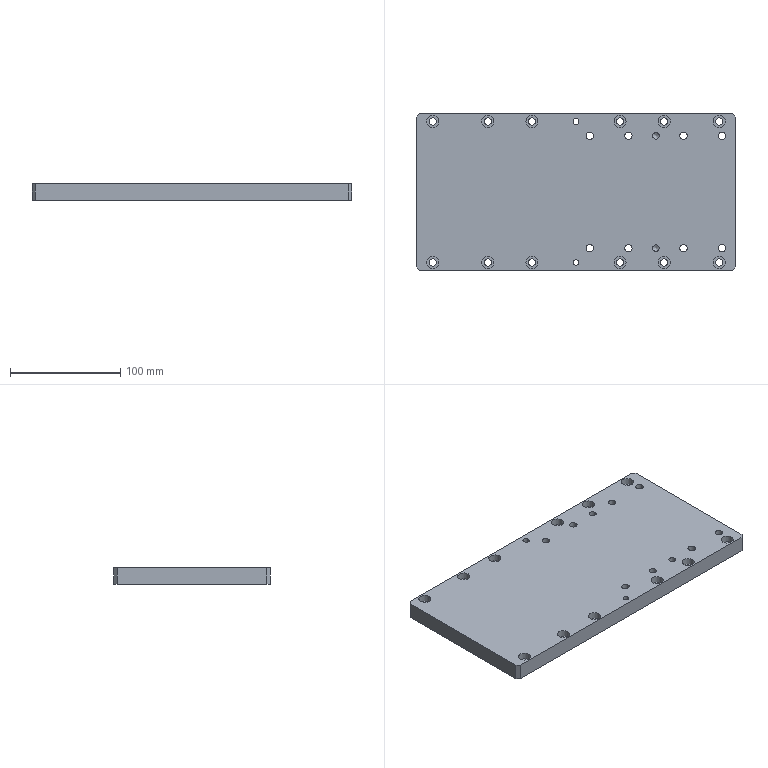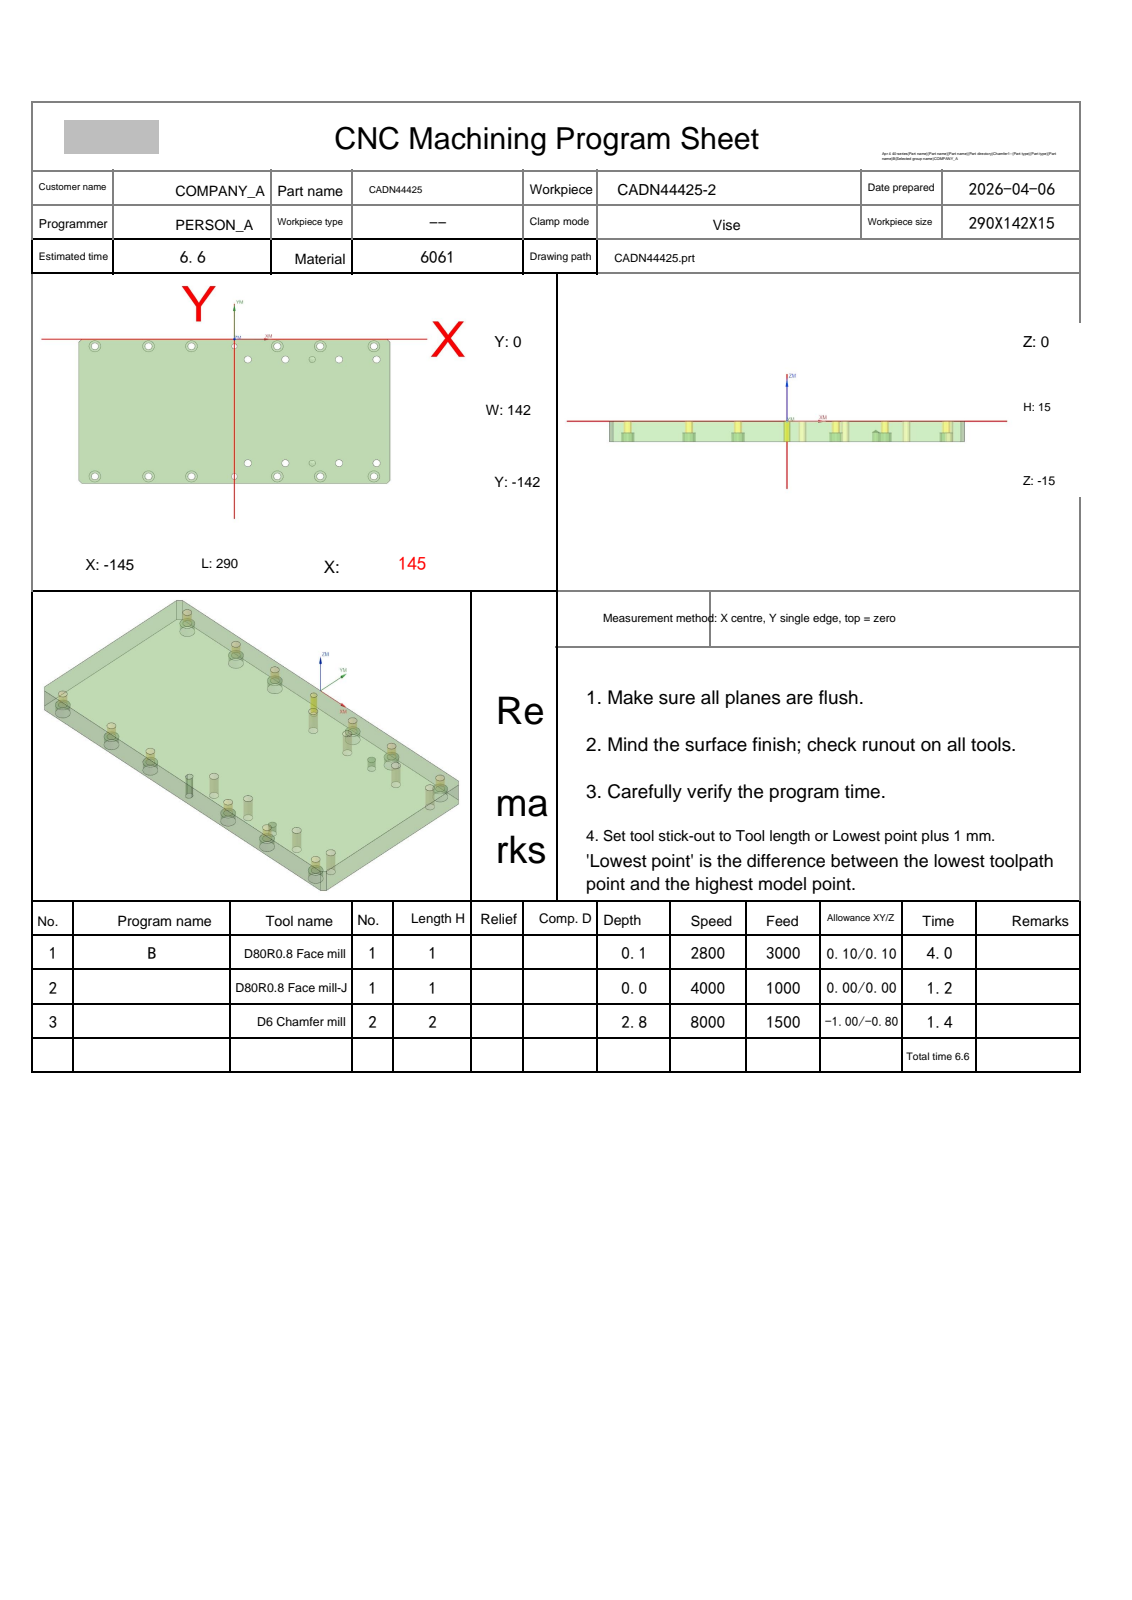NC program | NX | posted by the shop | part box 290 x 142 x 15 mm
Whole program:
%
O0001
(Machine time: 7.13 MIN)
(===Total Tool:2===)
(T1=D80R0.8 Face mill D=80.  R=0.8  D-  H01 Z=0.    )
(T2=D6 Chamfer mill   D=6.   R=0.   D-  H02 Z=-2.8  )
G80 G90 G17 G49 G40
G91 G28 Z0
M01
N1 T01 M06
(D80R0.8 Face mill  D=80. R=0.8 H=01 ce=0.10 di=0.10)
G00 G90 G54 X197.097 Y-118.097 M03 S2800
G43 H01 Z20.
M08
Z6.011
G01 Z4.011 F3000.
X185.097
X-177.897
G02 X-185.097 Y-110.897 I0.0 J7.2
G01 Y-82.68
G02 X-177.097 Y-74.68 I8. J0.0
G01 X177.897
G03 X185.097 Y-67.48 I0.0 J7.2
G01 Y-39.263
G03 X177.097 Y-31.263 I-8. J0.0
G01 X-185.097
X-197.097
Z6.011
G00 X197.097 Y-118.097
Z5.522
G01 Z3.522
X185.097
X-177.897
G02 X-185.097 Y-110.897 I0.0 J7.2
G01 Y-82.68
G02 X-177.097 Y-74.68 I8. J0.0
G01 X177.897
G03 X185.097 Y-67.48 I0.0 J7.2
G01 Y-39.263
G03 X177.097 Y-31.263 I-8. J0.0
G01 X-185.097
X-197.097
Z5.522
G00 X197.097 Y-118.097
Z5.033
G01 Z3.033
X185.097
X-177.897
G02 X-185.097 Y-110.897 I0.0 J7.2
G01 Y-82.68
G02 X-177.097 Y-74.68 I8. J0.0
G01 X177.897
G03 X185.097 Y-67.48 I0.0 J7.2
G01 Y-39.263
G03 X177.097 Y-31.263 I-8. J0.0
G01 X-185.097
X-197.097
Z5.033
G00 X197.097 Y-118.097
Z4.544
G01 Z2.544
X185.097
X-177.897
G02 X-185.097 Y-110.897 I0.0 J7.2
G01 Y-82.68
G02 X-177.097 Y-74.68 I8. J0.0
G01 X177.897
G03 X185.097 Y-67.48 I0.0 J7.2
G01 Y-39.263
G03 X177.097 Y-31.263 I-8. J0.0
G01 X-185.097
X-197.097
Z4.544
G00 Z20.
X197.097 Y-118.097
Z4.056
G01 Z2.056
X185.097
X-177.897
G02 X-185.097 Y-110.897 I0.0 J7.2
G01 Y-82.68
G02 X-177.097 Y-74.68 I8. J0.0
G01 X177.897
G03 X185.097 Y-67.48 I0.0 J7.2
G01 Y-39.263
G03 X177.097 Y-31.263 I-8. J0.0
G01 X-185.097
X-197.097
Z4.056
G00 Z20.
X197.097 Y-118.097
Z3.567
G01 Z1.567
X185.097
X-177.897
G02 X-185.097 Y-110.897 I0.0 J7.2
G01 Y-82.68
G02 X-177.097 Y-74.68 I8. J0.0
G01 X177.897
G03 X185.097 Y-67.48 I0.0 J7.2
G01 Y-39.263
G03 X177.097 Y-31.263 I-8. J0.0
G01 X-185.097
X-197.097
Z3.567
G00 Z20.
X197.097 Y-118.097
Z3.078
G01 Z1.078
X185.097
X-177.897
G02 X-185.097 Y-110.897 I0.0 J7.2
G01 Y-82.68
G02 X-177.097 Y-74.68 I8. J0.0
G01 X177.897
G03 X185.097 Y-67.48 I0.0 J7.2
G01 Y-39.263
G03 X177.097 Y-31.263 I-8. J0.0
G01 X-185.097
X-197.097
Z3.078
G00 Z20.
X197.097 Y-118.097
Z2.589
G01 Z.589
X185.097
X-177.897
G02 X-185.097 Y-110.897 I0.0 J7.2
G01 Y-82.68
G02 X-177.097 Y-74.68 I8. J0.0
G01 X177.897
G03 X185.097 Y-67.48 I0.0 J7.2
G01 Y-39.263
G03 X177.097 Y-31.263 I-8. J0.0
G01 X-185.097
X-197.097
Z2.589
G00 Z20.
X197.097 Y-118.097
Z2.1
G01 Z.1
X185.097
X-177.897
G02 X-185.097 Y-110.897 I0.0 J7.2
G01 Y-82.68
G02 X-177.097 Y-74.68 I8. J0.0
G01 X177.897
G03 X185.097 Y-67.48 I0.0 J7.2
G01 Y-39.263
G03 X177.097 Y-31.263 I-8. J0.0
G01 X-185.097
X-197.097
Z2.1
G00 Z20.
G91 G28 Z0.0
M05
M09
G91 G28 Z0.0
M01
N2 T01 M06
(D80R0.8 Face mill-J  D=80. R=0.8 H=01 ce=0.00 di=0.00)
G00 G90 G54 X196.999 Y-117.999 M03 S4000
G43 H01 Z20.
M08
Z2.
G01 Z0.0 F1000.
X184.999
X-177.799
G02 X-184.999 Y-110.799 I0.0 J7.2
G01 Y-82.68
G02 X-176.999 Y-74.68 I8. J0.0
G01 X177.799
G03 X184.999 Y-67.48 I0.0 J7.2
G01 Y-39.361
G03 X176.999 Y-31.361 I-8. J0.0
G01 X-184.999
X-196.999
Z2.
G00 Z20.
G91 G28 Z0.0
M05
M09
G91 G28 Z0.0
M01
N3 T02 M06
(D6 Chamfer mill  D=6. R=0. H=02 ce=0.00 di=0.00)
G00 G90 G54 X0.0 Y-7. M03 S8000
G43 H02 Z20.
M08
G98 G81 X0.0 Y-7. Z-2.8 R3. F1000.
G80
G00 Z20.
G00 G90 X129.493 Y-133.913 M03 S8000
Z20.
Z-.9
G01 Z-1.4 F1200.
X129.3 Y-133.5
G03 X127.8 Y-135. I0.0 J-1.5
X130. Y-137.2 I2.2 J0.0
X132.2 Y-135. I0.0 J2.2
X130. Y-132.8 I-2.2 J0.0
X127.8 Y-135. I0.0 J-2.2
X129.3 Y-136.5 I1.5 J0.0
G01 X129.493 Y-136.087
Z-.9
G00 Z20.
X79.493 Y-133.913
Z-.9
G01 Z-1.4
X79.3 Y-133.5
G03 X77.8 Y-135. I0.0 J-1.5
X80. Y-137.2 I2.2 J0.0
X82.2 Y-135. I0.0 J2.2
X80. Y-132.8 I-2.2 J0.0
X77.8 Y-135. I0.0 J-2.2
X79.3 Y-136.5 I1.5 J0.0
G01 X79.493 Y-136.087
Z-.9
G00 Z20.
X39.493 Y-133.913
Z-.9
G01 Z-1.4
X39.3 Y-133.5
G03 X37.8 Y-135. I0.0 J-1.5
X40. Y-137.2 I2.2 J0.0
X42.2 Y-135. I0.0 J2.2
X40. Y-132.8 I-2.2 J0.0
X37.8 Y-135. I0.0 J-2.2
X39.3 Y-136.5 I1.5 J0.0
G01 X39.493 Y-136.087
Z-.9
G00 Z20.
X-40.507 Y-133.913
Z-.9
G01 Z-1.4
X-40.7 Y-133.5
G03 X-42.2 Y-135. I0.0 J-1.5
X-40. Y-137.2 I2.2 J0.0
X-37.8 Y-135. I0.0 J2.2
X-40. Y-132.8 I-2.2 J0.0
X-42.2 Y-135. I0.0 J-2.2
X-40.7 Y-136.5 I1.5 J0.0
G01 X-40.507 Y-136.087
Z-.9
G00 Z20.
X-80.507 Y-133.913
Z-.9
G01 Z-1.4
X-80.7 Y-133.5
G03 X-82.2 Y-135. I0.0 J-1.5
X-80. Y-137.2 I2.2 J0.0
X-77.8 Y-135. I0.0 J2.2
X-80. Y-132.8 I-2.2 J0.0
X-82.2 Y-135. I0.0 J-2.2
X-80.7 Y-136.5 I1.5 J0.0
G01 X-80.507 Y-136.087
Z-.9
G00 Z20.
X-130.507 Y-133.913
Z-.9
G01 Z-1.4
X-130.7 Y-133.5
G03 X-132.2 Y-135. I0.0 J-1.5
X-130. Y-137.2 I2.2 J0.0
X-127.8 Y-135. I0.0 J2.2
X-130. Y-132.8 I-2.2 J0.0
X-132.2 Y-135. I0.0 J-2.2
X-130.7 Y-136.5 I1.5 J0.0
G01 X-130.507 Y-136.087
Z-.9
G00 Z20.
Y-5.913
Z-.9
G01 Z-1.4
X-130.7 Y-5.5
G03 X-132.2 Y-7. I0.0 J-1.5
X-130. Y-9.2 I2.2 J0.0
X-127.8 Y-7. I0.0 J2.2
X-130. Y-4.8 I-2.2 J0.0
X-132.2 Y-7. I0.0 J-2.2
X-130.7 Y-8.5 I1.5 J0.0
G01 X-130.507 Y-8.087
Z-.9
G00 Z20.
X-80.507 Y-5.913
Z-.9
G01 Z-1.4
X-80.7 Y-5.5
G03 X-82.2 Y-7. I0.0 J-1.5
X-80. Y-9.2 I2.2 J0.0
X-77.8 Y-7. I0.0 J2.2
X-80. Y-4.8 I-2.2 J0.0
X-82.2 Y-7. I0.0 J-2.2
X-80.7 Y-8.5 I1.5 J0.0
G01 X-80.507 Y-8.087
Z-.9
G00 Z20.
X-40.507 Y-5.913
Z-.9
G01 Z-1.4
X-40.7 Y-5.5
G03 X-42.2 Y-7. I0.0 J-1.5
X-40. Y-9.2 I2.2 J0.0
X-37.8 Y-7. I0.0 J2.2
X-40. Y-4.8 I-2.2 J0.0
X-42.2 Y-7. I0.0 J-2.2
X-40.7 Y-8.5 I1.5 J0.0
G01 X-40.507 Y-8.087
Z-.9
G00 Z20.
X39.493 Y-5.913
Z-.9
G01 Z-1.4
X39.3 Y-5.5
G03 X37.8 Y-7. I0.0 J-1.5
X40. Y-9.2 I2.2 J0.0
X42.2 Y-7. I0.0 J2.2
X40. Y-4.8 I-2.2 J0.0
X37.8 Y-7. I0.0 J-2.2
X39.3 Y-8.5 I1.5 J0.0
G01 X39.493 Y-8.087
Z-.9
G00 Z20.
X79.493 Y-5.913
Z-.9
G01 Z-1.4
X79.3 Y-5.5
G03 X77.8 Y-7. I0.0 J-1.5
X80. Y-9.2 I2.2 J0.0
X82.2 Y-7. I0.0 J2.2
X80. Y-4.8 I-2.2 J0.0
X77.8 Y-7. I0.0 J-2.2
X79.3 Y-8.5 I1.5 J0.0
G01 X79.493 Y-8.087
Z-.9
G00 Z20.
X129.493 Y-5.913
Z-.9
G01 Z-1.4
X129.3 Y-5.5
G03 X127.8 Y-7. I0.0 J-1.5
X130. Y-9.2 I2.2 J0.0
X132.2 Y-7. I0.0 J2.2
X130. Y-4.8 I-2.2 J0.0
X127.8 Y-7. I0.0 J-2.2
X129.3 Y-8.5 I1.5 J0.0
G01 X129.493 Y-8.087
Z-.9
G00 Z20.
G00 G90 X132.5 Y-120. M03 S8000
Z20.
Z-.9
G01 Z-1.4 F600.
Y-119.
G03 X129.5 Y-122. I0.0 J-3.
X132.5 Y-125. I3. J0.0
X135.5 Y-122. I0.0 J3.
X132.5 Y-119. I-3. J0.0
X129.5 Y-122. I0.0 J-3.
X132.5 Y-125. I3. J0.0
G01 Y-124.
Z-.9
G00 Z20.
X97.5 Y-120.
Z-.9
G01 Z-1.4
Y-119.
G03 X94.5 Y-122. I0.0 J-3.
X97.5 Y-125. I3. J0.0
X100.5 Y-122. I0.0 J3.
X97.5 Y-119. I-3. J0.0
X94.5 Y-122. I0.0 J-3.
X97.5 Y-125. I3. J0.0
G01 Y-124.
Z-.9
G00 Z20.
X47.5 Y-120.
Z-.9
G01 Z-1.4
Y-119.
G03 X44.5 Y-122. I0.0 J-3.
X47.5 Y-125. I3. J0.0
X50.5 Y-122. I0.0 J3.
X47.5 Y-119. I-3. J0.0
X44.5 Y-122. I0.0 J-3.
X47.5 Y-125. I3. J0.0
G01 Y-124.
Z-.9
G00 Z20.
X12.5 Y-120.
Z-.9
G01 Z-1.4
Y-119.
G03 X9.5 Y-122. I0.0 J-3.
X12.5 Y-125. I3. J0.0
X15.5 Y-122. I0.0 J3.
X12.5 Y-119. I-3. J0.0
X9.5 Y-122. I0.0 J-3.
X12.5 Y-125. I3. J0.0
G01 Y-124.
Z-.9
G00 Z20.
Y-18.
Z-.9
G01 Z-1.4
Y-17.
G03 X9.5 Y-20. I0.0 J-3.
X12.5 Y-23. I3. J0.0
X15.5 Y-20. I0.0 J3.
X12.5 Y-17. I-3. J0.0
X9.5 Y-20. I0.0 J-3.
X12.5 Y-23. I3. J0.0
G01 Y-22.
Z-.9
G00 Z20.
X47.5 Y-18.
Z-.9
G01 Z-1.4
Y-17.
G03 X44.5 Y-20. I0.0 J-3.
X47.5 Y-23. I3. J0.0
X50.5 Y-20. I0.0 J3.
X47.5 Y-17. I-3. J0.0
X44.5 Y-20. I0.0 J-3.
X47.5 Y-23. I3. J0.0
G01 Y-22.
Z-.9
G00 Z20.
X97.5 Y-18.
Z-.9
G01 Z-1.4
Y-17.
G03 X94.5 Y-20. I0.0 J-3.
X97.5 Y-23. I3. J0.0
X100.5 Y-20. I0.0 J3.
X97.5 Y-17. I-3. J0.0
X94.5 Y-20. I0.0 J-3.
X97.5 Y-23. I3. J0.0
G01 Y-22.
Z-.9
G00 Z20.
X132.5 Y-18.
Z-.9
G01 Z-1.4
Y-17.
G03 X129.5 Y-20. I0.0 J-3.
X132.5 Y-23. I3. J0.0
X135.5 Y-20. I0.0 J3.
X132.5 Y-17. I-3. J0.0
X129.5 Y-20. I0.0 J-3.
X132.5 Y-23. I3. J0.0
G01 Y-22.
Z-.9
G00 Z20.
G00 G90 X133.046 Y.7 M03 S7000
Z20.
Z2.5
G01 X141.953 Z-.742 F1500.
X142.16 Y.662 Z-.819
X142.355 Y.581 Z-.895
X142.528 Y.462 Z-.972
X142.583 Y.407 Z-1.
X145.407 Y-2.417
G02 X145.7 Y-3.124 I-.707 J-.707
G01 Y-138.876
G02 X145.407 Y-139.583 I-1. J0.0
G01 X142.583 Y-142.407
G02 X141.876 Y-142.7 I-.707 J.707
G01 X-141.876
G02 X-142.583 Y-142.407 I0.0 J1.
G01 X-145.407 Y-139.583
G02 X-145.7 Y-138.876 I.707 J.707
G01 Y-3.124
G02 X-145.407 Y-2.417 I1. J0.0
G01 X-142.583 Y.407
G02 X-141.876 Y.7 I.707 J-.707
G01 X141.876
G02 X142.583 Y.407 I0.0 J-1.
G01 X142.936 Y.054
Z1.5
G00 Z20.
X.836 Y-137.091
Z2.5
G01 X.931 Y-137.044 Z2.461
X1.168 Y-136.874 Z2.355
X1.374 Y-136.668 Z2.249
X1.544 Y-136.431 Z2.143
X1.674 Y-136.171 Z2.037
X1.76 Y-135.892 Z1.931
X1.8 Y-135.604 Z1.825
Y-134.396 Z1.386
X1.76 Y-134.108 Z1.28
X1.674 Y-133.829 Z1.174
X1.544 Y-133.569 Z1.068
X1.374 Y-133.332 Z.962
X1.168 Y-133.126 Z.856
X.931 Y-132.956 Z.75
X.671 Y-132.826 Z.644
X.392 Y-132.74 Z.538
X.104 Y-132.7 Z.432
X-.104 Z.356
X-.392 Y-132.74 Z.25
X-.671 Y-132.826 Z.144
X-.931 Y-132.956 Z.038
X-1.168 Y-133.126 Z-.068
X-1.374 Y-133.332 Z-.174
X-1.544 Y-133.569 Z-.28
X-1.674 Y-133.829 Z-.386
X-1.76 Y-134.108 Z-.492
X-1.8 Y-134.396 Z-.598
Y-135.5 Z-1.
G03 X0.0 Y-137.3 I1.8 J0.0
X1.8 Y-135.5 I0.0 J1.8
G01 Y-134.5
G03 X0.0 Y-132.7 I-1.8 J0.0
X-1.8 Y-134.5 I0.0 J-1.8
G01 Y-135.5
G03 X-1.731 Y-135.994 I1.8 J0.0
G01 Z1.5
G00 Z20.
M05
M09
G91 G28 Z0.0
G91 G28 Y0.0
M30
%